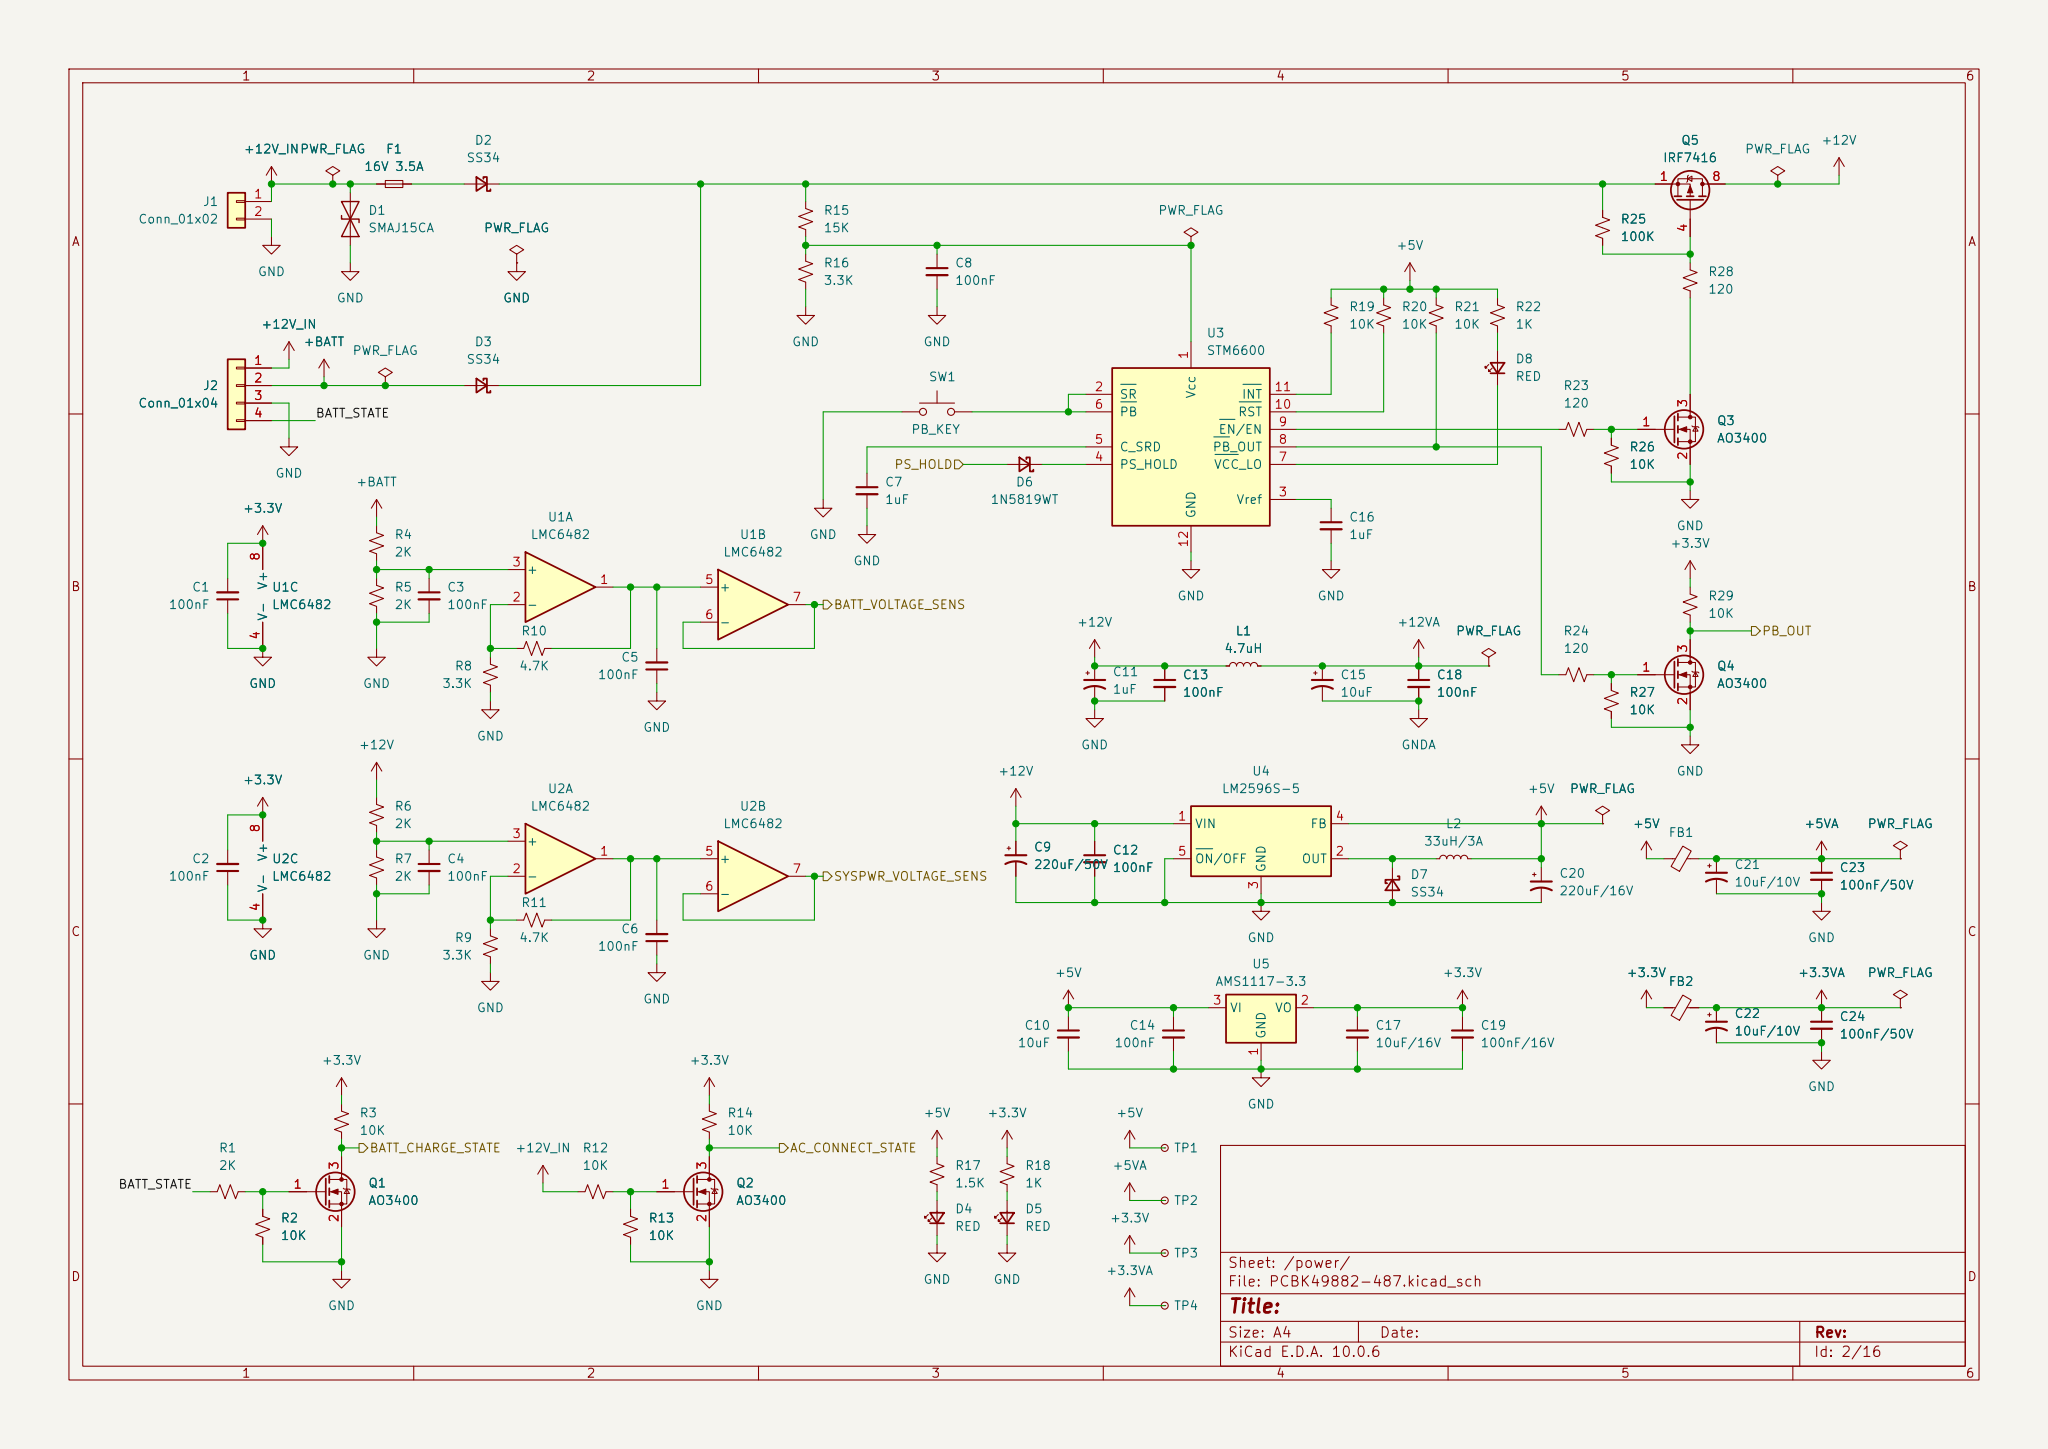Circuit board | KiCad | 536 parts | 438 nets | one sheet of the schematic
Parts on this sheet (reference | value | footprint):
C1
C11 | 1uF | Capacitor_Tantalum_SMD:CP_EIA-3216-18_Kemet-A
C12
C13
C14
C15 | 10uF | Capacitor_Tantalum_SMD:CP_EIA-3216-18_Kemet-A
C16 | 1uF | Capacitor_SMD:C_0603_1608Metric
C17 | 10uF/16V | Capacitor_SMD:C_0805_2012Metric
C18 | 100nF | Capacitor_SMD:C_0603_1608Metric
C19 | 100nF/16V | Capacitor_SMD:C_0603_1608Metric
C2
C20 | 220uF/16V | Capacitor_SMD:CP_Elec_6.3x5.4
C21 | 10uF/10V | Capacitor_Tantalum_SMD:CP_EIA-3528-21_Kemet-B
C22 | 10uF/10V | Capacitor_Tantalum_SMD:CP_EIA-3528-21_Kemet-B
C23 | 100nF/50V | Capacitor_SMD:C_0603_1608Metric
C24 | 100nF/50V | Capacitor_SMD:C_0603_1608Metric
C3
C4
C5
C6
C7 | 1uF | Capacitor_SMD:C_0603_1608Metric
C8 | 100nF | Capacitor_SMD:C_0603_1608Metric
C9 | 220uF/50V | Capacitor_SMD:CP_Elec_6.3x7.7
D1 | SMAJ15CA | Diode_SMD:D_SMA
D2 | SS34 | Diode_SMD:D_SMA
D3 | SS34 | Diode_SMD:D_SMA
D6 | 1N5819WT | Diode_SMD:D_SOD-523
D7 | SS34 | Diode_SMD:D_SMA
F1 | 16V 3.5A | Fuse:Fuse_1812_4532Metric
FB1 | 100ohm @100MHz max. 4000mA | Inductor_SMD:L_0805_2012Metric
FB2 | 100ohm @100MHz max. 4000mA | Inductor_SMD:L_0805_2012Metric
J1 | Conn_01x02 | Connector_Molex:Molex_KK-396_5273-02A_1x02_P3.96mm_Vertical
J2 | Conn_01x04 | Connector_Molex:Molex_KK-396_5273-04A_1x04_P3.96mm_Vertical
L1 | 4.7uH | Inductor_SMD:L_Sunlord_SWPA4030S
L2 | 33uH/3A | Inductor_SMD:L_Sunlord_SWRB1207S
Q5 | IRF7416 | Package_SO:SOIC-8_3.9x4.9mm_P1.27mm
R1 | 2K | Resistor_SMD:R_0603_1608Metric
R10 | 4.7K | Resistor_SMD:R_0603_1608Metric
R11 | 4.7K | Resistor_SMD:R_0603_1608Metric
R12
R13
R15 | 15K | Resistor_SMD:R_0603_1608Metric
R16 | 3.3K | Resistor_SMD:R_0603_1608Metric
R17 | 1.5K | Resistor_SMD:R_0603_1608Metric
R18 | 1K | Resistor_SMD:R_0603_1608Metric
R19
R20
R21
R22 | 1K | Resistor_SMD:R_0603_1608Metric
R23 | 120 | Resistor_SMD:R_0603_1608Metric
R24 | 120 | Resistor_SMD:R_0603_1608Metric
R25 | 100K | Resistor_SMD:R_0603_1608Metric
R26 | 10K | Resistor_SMD:R_0603_1608Metric
R27 | 10K | Resistor_SMD:R_0603_1608Metric
R28 | 120 | Resistor_SMD:R_0603_1608Metric
R29
R4
R6
R7
R8 | 3.3K | Resistor_SMD:R_0603_1608Metric
R9 | 3.3K | Resistor_SMD:R_0603_1608Metric
SW1 | PB_KEY | Button_Switch_SMD:SW_Push_1P1T_NO_6x6mm_H9.5mm
TP1
TP2
TP3
TP4
U3 | STM6600 | Package_DFN_QFN:TDFN-12_2x3mm_P0.5mm
U4 | LM2596S-5 | Package_TO_SOT_SMD:TO-263-5_TabPin3
U5 | AMS1117-3.3 | Package_TO_SOT_SMD:SOT-223-3_TabPin2
Nets of these parts (net: part-pin ...):
+3.3V: C1-2 C2-2 C17-1 C19-1 FB2-1 R18-1 R29-2 TP3-1 U5-2
+3.3VA: C22-1 C24-1 FB2-2 TP4-1
+5V: C14-1 C20-1 FB1-1 L2-2 R17-1 R19-1 R20-1 R21-1 R22-1 TP1-1 U4-4 U5-3
+5VA: C21-1 C23-1 FB1-2 TP2-1
+12V: C9-1 C11-1 C12-1 C13-1 L1-1 Q5-5 Q5-6 Q5-7 Q5-8 R6-2 U4-1
+12VA: C15-1 C18-1 L1-2
+12V_IN: D1-2 F1-1 J1-1 J2-1 R12-1
+BATT: D3-2 J2-2 R4-2
/core_board_b2b/PG10{slash}PB_OUT: R29-1
/core_board_b2b/PG11{slash}PS_HOLD: D6-2
/power/BATT_STATE: J2-4 R1-1
GND: C1-1 C2-1 C3-2 C4-2 C5-1 C6-1 C7-2 C8-2 C9-2 C11-2 C12-2 C13-2 C14-2 C16-2 C17-2 C19-2 C20-2 C21-2 C22-2 C23-2 C24-2 D1-1 D7-2 J1-2 J2-3 R7-1 R8-1 R9-1 R13-1 R16-2 R26-1 R27-1 SW1-1 U3-12 U4-3 U4-5 U5-1
GNDA: C15-2 C18-2
Net-(D2-A): D2-2 F1-2
Net-(D2-K): D2-1 D3-1 Q5-1 Q5-2 Q5-3 R15-1 R25-1
Net-(D4-A): R17-2
Net-(D5-A): R18-2
Net-(D6-K): D6-1 U3-4
Net-(D7-K): D7-1 L2-1 U4-2
Net-(D8-A): R22-2
Net-(D8-K): U3-7
Net-(Q1-G): R1-2
Net-(Q2-G): R12-2 R13-2
Net-(Q3-D): R28-2
Net-(Q3-G): R23-2 R26-2
Net-(Q4-G): R24-2 R27-2
Net-(Q5-G): Q5-4 R25-2 R28-1
Net-(U1A-+): C3-1 R4-1
Net-(U1A--): R8-2 R10-1
Net-(U1B-+): C5-2 R10-2
Net-(U2A-+): C4-1 R6-1 R7-2
Net-(U2A--): R9-2 R11-1
Net-(U2B-+): C6-2 R11-2
Net-(U3-C_SRD): C7-1 U3-5
Net-(U3-Vcc): C8-1 R15-2 R16-1 U3-1
Net-(U3-Vref): C16-1 U3-3
Net-(U3-~{EN}{slash}EN): R23-1 U3-9
Net-(U3-~{INT}): R19-2 U3-11
Net-(U3-~{PB}): SW1-2 U3-2 U3-6
Net-(U3-~{PB}_OUT): R21-2 R24-1 U3-8
Net-(U3-~{RST}): R20-2 U3-10